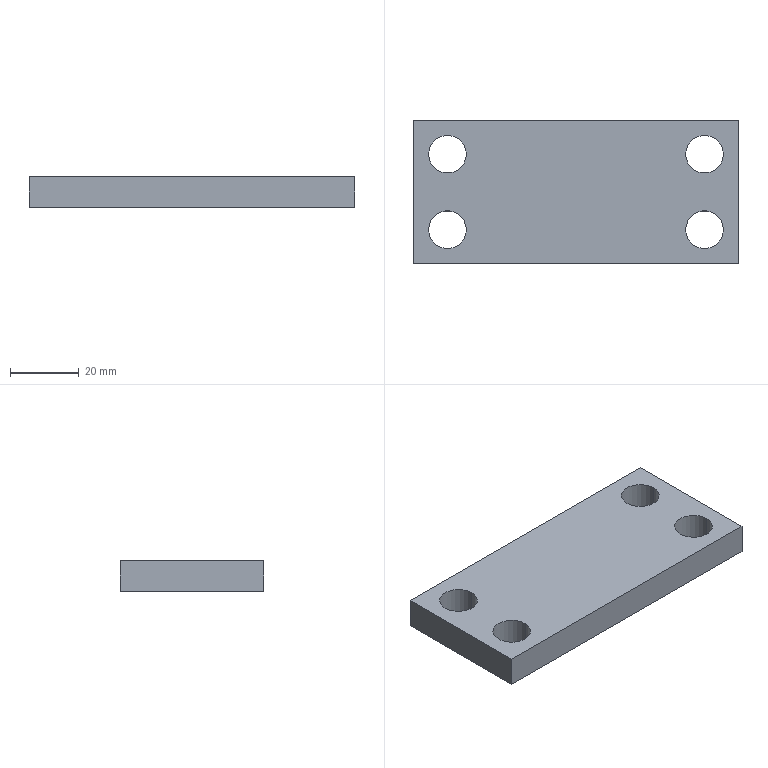Part | STEP file | 0244_203_Spacer | 1 solid | 14 faces | box 95 x 42 x 9 mm | volume 32489 mm3 | cylinder 8 | plane 6 | commonest cylinder face diameters 11 x8
STEP:
#1=CARTESIAN_POINT('',(0.,0.,0.));
#2=DIRECTION('',(0.,0.,1.));
#3=DIRECTION('',(1.,0.,0.));
#4=AXIS2_PLACEMENT_3D('',#1,#2,#3);
#5=CARTESIAN_POINT('',(43.,32.,0.));
#6=VERTEX_POINT('',#5);
#7=CARTESIAN_POINT('',(43.,32.,9.));
#8=VERTEX_POINT('',#7);
#9=CARTESIAN_POINT('',(43.,32.,9.));
#10=DIRECTION('',(0.,0.,1.));
#11=VECTOR('',#10,1.);
#12=LINE('',#9,#11);
#13=CARTESIAN_POINT('',(37.5,32.,9.));
#14=DIRECTION('',(0.,0.,1.));
#15=DIRECTION('',(1.,0.,0.));
#16=AXIS2_PLACEMENT_3D('',#13,#14,#15);
#17=CYLINDRICAL_SURFACE('',#16,5.5);
#18=CARTESIAN_POINT('',(6.283,0.));
#19=DIRECTION('',(0.,1.));
#20=VECTOR('',#19,1.);
#21=LINE('',#18,#20);
#22=(GEOMETRIC_REPRESENTATION_CONTEXT(2)PARAMETRIC_REPRESENTATION_CONTEXT()REPRESENTATION_CONTEXT('',''));
#23=DEFINITIONAL_REPRESENTATION('',(#21),#22);
#24=PCURVE('',#17,#23);
#25=CARTESIAN_POINT('',(37.5,32.,9.));
#26=DIRECTION('',(0.,0.,1.));
#27=DIRECTION('',(1.,0.,0.));
#28=AXIS2_PLACEMENT_3D('',#25,#26,#27);
#29=CYLINDRICAL_SURFACE('',#28,5.5);
#30=CARTESIAN_POINT('',(0.,0.));
#31=DIRECTION('',(0.,1.));
#32=VECTOR('',#31,1.);
#33=LINE('',#30,#32);
#34=(GEOMETRIC_REPRESENTATION_CONTEXT(2)PARAMETRIC_REPRESENTATION_CONTEXT()REPRESENTATION_CONTEXT('',''));
#35=DEFINITIONAL_REPRESENTATION('',(#33),#34);
#36=PCURVE('',#29,#35);
#37=SURFACE_CURVE('',#12,(#24,#36),.PCURVE_S1.);
#38=EDGE_CURVE('',#6,#8,#37,.T.);
#39=ORIENTED_EDGE('',*,*,#38,.T.);
#40=CARTESIAN_POINT('',(32.,32.,9.));
#41=VERTEX_POINT('',#40);
#42=CARTESIAN_POINT('',(37.5,32.,9.));
#43=DIRECTION('',(0.,0.,1.));
#44=DIRECTION('',(1.,0.,0.));
#45=AXIS2_PLACEMENT_3D('',#42,#43,#44);
#46=CIRCLE('',#45,5.5);
#47=CARTESIAN_POINT('',(0.,0.));
#48=DIRECTION('',(1.,0.));
#49=VECTOR('',#48,1.);
#50=LINE('',#47,#49);
#51=(GEOMETRIC_REPRESENTATION_CONTEXT(2)PARAMETRIC_REPRESENTATION_CONTEXT()REPRESENTATION_CONTEXT('',''));
#52=DEFINITIONAL_REPRESENTATION('',(#50),#51);
#53=PCURVE('',#17,#52);
#54=CARTESIAN_POINT('',(-47.5,42.,9.));
#55=DIRECTION('',(0.,0.,-1.));
#56=DIRECTION('',(-1.,0.,0.));
#57=AXIS2_PLACEMENT_3D('',#54,#55,#56);
#58=PLANE('',#57);
#59=CARTESIAN_POINT('',(-90.5,-10.));
#60=CARTESIAN_POINT('',(-90.5,-0.4737));
#61=CARTESIAN_POINT('',(-82.25,-5.237));
#62=CARTESIAN_POINT('',(-74.,-10.));
#63=CARTESIAN_POINT('',(-82.25,-14.763));
#64=CARTESIAN_POINT('',(-90.5,-19.526));
#65=CARTESIAN_POINT('',(-90.5,-10.));
#66=(BOUNDED_CURVE()B_SPLINE_CURVE(2,(#59,#60,#61,#62,#63,#64,#65),.UNSPECIFIED.,.T.,.F.)B_SPLINE_CURVE_WITH_KNOTS((1,2,2,2,2,1),(-2.094,0.,2.094,4.189,6.283,8.378),.UNSPECIFIED.)CURVE()GEOMETRIC_REPRESENTATION_ITEM()RATIONAL_B_SPLINE_CURVE((1.,0.5,1.,0.5,1.,0.5,1.))REPRESENTATION_ITEM(''));
#67=(GEOMETRIC_REPRESENTATION_CONTEXT(2)PARAMETRIC_REPRESENTATION_CONTEXT()REPRESENTATION_CONTEXT('',''));
#68=DEFINITIONAL_REPRESENTATION('',(#66),#67);
#69=PCURVE('',#58,#68);
#70=SURFACE_CURVE('',#46,(#53,#69),.PCURVE_S1.);
#71=EDGE_CURVE('',#41,#8,#70,.T.);
#72=ORIENTED_EDGE('',*,*,#71,.F.);
#73=CARTESIAN_POINT('',(32.,32.,0.));
#74=VERTEX_POINT('',#73);
#75=CARTESIAN_POINT('',(32.,32.,9.));
#76=DIRECTION('',(0.,0.,1.));
#77=VECTOR('',#76,1.);
#78=LINE('',#75,#77);
#79=CARTESIAN_POINT('',(3.142,0.));
#80=DIRECTION('',(0.,1.));
#81=VECTOR('',#80,1.);
#82=LINE('',#79,#81);
#83=(GEOMETRIC_REPRESENTATION_CONTEXT(2)PARAMETRIC_REPRESENTATION_CONTEXT()REPRESENTATION_CONTEXT('',''));
#84=DEFINITIONAL_REPRESENTATION('',(#82),#83);
#85=PCURVE('',#17,#84);
#86=CARTESIAN_POINT('',(3.142,0.));
#87=DIRECTION('',(0.,1.));
#88=VECTOR('',#87,1.);
#89=LINE('',#86,#88);
#90=(GEOMETRIC_REPRESENTATION_CONTEXT(2)PARAMETRIC_REPRESENTATION_CONTEXT()REPRESENTATION_CONTEXT('',''));
#91=DEFINITIONAL_REPRESENTATION('',(#89),#90);
#92=PCURVE('',#29,#91);
#93=SURFACE_CURVE('',#78,(#85,#92),.PCURVE_S1.);
#94=EDGE_CURVE('',#74,#41,#93,.T.);
#95=ORIENTED_EDGE('',*,*,#94,.F.);
#96=CARTESIAN_POINT('',(37.5,32.,0.));
#97=DIRECTION('',(0.,0.,1.));
#98=DIRECTION('',(1.,0.,0.));
#99=AXIS2_PLACEMENT_3D('',#96,#97,#98);
#100=CIRCLE('',#99,5.5);
#101=CARTESIAN_POINT('',(0.,-9.));
#102=DIRECTION('',(1.,0.));
#103=VECTOR('',#102,1.);
#104=LINE('',#101,#103);
#105=(GEOMETRIC_REPRESENTATION_CONTEXT(2)PARAMETRIC_REPRESENTATION_CONTEXT()REPRESENTATION_CONTEXT('',''));
#106=DEFINITIONAL_REPRESENTATION('',(#104),#105);
#107=PCURVE('',#17,#106);
#108=CARTESIAN_POINT('',(-47.5,42.,0.));
#109=DIRECTION('',(0.,0.,-1.));
#110=DIRECTION('',(-1.,0.,0.));
#111=AXIS2_PLACEMENT_3D('',#108,#109,#110);
#112=PLANE('',#111);
#113=CARTESIAN_POINT('',(-90.5,-10.));
#114=CARTESIAN_POINT('',(-90.5,-0.4737));
#115=CARTESIAN_POINT('',(-82.25,-5.237));
#116=CARTESIAN_POINT('',(-74.,-10.));
#117=CARTESIAN_POINT('',(-82.25,-14.763));
#118=CARTESIAN_POINT('',(-90.5,-19.526));
#119=CARTESIAN_POINT('',(-90.5,-10.));
#120=(BOUNDED_CURVE()B_SPLINE_CURVE(2,(#113,#114,#115,#116,#117,#118,#119),.UNSPECIFIED.,.T.,.F.)B_SPLINE_CURVE_WITH_KNOTS((1,2,2,2,2,1),(-2.094,0.,2.094,4.189,6.283,8.378),.UNSPECIFIED.)CURVE()GEOMETRIC_REPRESENTATION_ITEM()RATIONAL_B_SPLINE_CURVE((1.,0.5,1.,0.5,1.,0.5,1.))REPRESENTATION_ITEM(''));
#121=(GEOMETRIC_REPRESENTATION_CONTEXT(2)PARAMETRIC_REPRESENTATION_CONTEXT()REPRESENTATION_CONTEXT('',''));
#122=DEFINITIONAL_REPRESENTATION('',(#120),#121);
#123=PCURVE('',#112,#122);
#124=SURFACE_CURVE('',#100,(#107,#123),.PCURVE_S1.);
#125=EDGE_CURVE('',#74,#6,#124,.T.);
#126=ORIENTED_EDGE('',*,*,#125,.T.);
#127=EDGE_LOOP('',(#39,#72,#95,#126));
#128=FACE_BOUND('',#127,.F.);
#129=ADVANCED_FACE('',(#128),#17,.F.);
#130=CARTESIAN_POINT('',(-32.,32.,0.));
#131=VERTEX_POINT('',#130);
#132=CARTESIAN_POINT('',(-32.,32.,9.));
#133=VERTEX_POINT('',#132);
#134=CARTESIAN_POINT('',(-32.,32.,9.));
#135=DIRECTION('',(0.,0.,1.));
#136=VECTOR('',#135,1.);
#137=LINE('',#134,#136);
#138=CARTESIAN_POINT('',(-37.5,32.,9.));
#139=DIRECTION('',(0.,0.,1.));
#140=DIRECTION('',(1.,0.,0.));
#141=AXIS2_PLACEMENT_3D('',#138,#139,#140);
#142=CYLINDRICAL_SURFACE('',#141,5.5);
#143=CARTESIAN_POINT('',(6.283,0.));
#144=DIRECTION('',(0.,1.));
#145=VECTOR('',#144,1.);
#146=LINE('',#143,#145);
#147=(GEOMETRIC_REPRESENTATION_CONTEXT(2)PARAMETRIC_REPRESENTATION_CONTEXT()REPRESENTATION_CONTEXT('',''));
#148=DEFINITIONAL_REPRESENTATION('',(#146),#147);
#149=PCURVE('',#142,#148);
#150=CARTESIAN_POINT('',(-37.5,32.,9.));
#151=DIRECTION('',(0.,0.,1.));
#152=DIRECTION('',(1.,0.,0.));
#153=AXIS2_PLACEMENT_3D('',#150,#151,#152);
#154=CYLINDRICAL_SURFACE('',#153,5.5);
#155=CARTESIAN_POINT('',(0.,0.));
#156=DIRECTION('',(0.,1.));
#157=VECTOR('',#156,1.);
#158=LINE('',#155,#157);
#159=(GEOMETRIC_REPRESENTATION_CONTEXT(2)PARAMETRIC_REPRESENTATION_CONTEXT()REPRESENTATION_CONTEXT('',''));
#160=DEFINITIONAL_REPRESENTATION('',(#158),#159);
#161=PCURVE('',#154,#160);
#162=SURFACE_CURVE('',#137,(#149,#161),.PCURVE_S1.);
#163=EDGE_CURVE('',#131,#133,#162,.T.);
#164=ORIENTED_EDGE('',*,*,#163,.T.);
#165=CARTESIAN_POINT('',(-43.,32.,9.));
#166=VERTEX_POINT('',#165);
#167=CARTESIAN_POINT('',(-37.5,32.,9.));
#168=DIRECTION('',(0.,0.,1.));
#169=DIRECTION('',(1.,0.,0.));
#170=AXIS2_PLACEMENT_3D('',#167,#168,#169);
#171=CIRCLE('',#170,5.5);
#172=CARTESIAN_POINT('',(0.,0.));
#173=DIRECTION('',(1.,0.));
#174=VECTOR('',#173,1.);
#175=LINE('',#172,#174);
#176=(GEOMETRIC_REPRESENTATION_CONTEXT(2)PARAMETRIC_REPRESENTATION_CONTEXT()REPRESENTATION_CONTEXT('',''));
#177=DEFINITIONAL_REPRESENTATION('',(#175),#176);
#178=PCURVE('',#142,#177);
#179=CARTESIAN_POINT('',(-15.5,-10.));
#180=CARTESIAN_POINT('',(-15.5,-0.4737));
#181=CARTESIAN_POINT('',(-7.25,-5.237));
#182=CARTESIAN_POINT('',(1.,-10.));
#183=CARTESIAN_POINT('',(-7.25,-14.763));
#184=CARTESIAN_POINT('',(-15.5,-19.526));
#185=CARTESIAN_POINT('',(-15.5,-10.));
#186=(BOUNDED_CURVE()B_SPLINE_CURVE(2,(#179,#180,#181,#182,#183,#184,#185),.UNSPECIFIED.,.T.,.F.)B_SPLINE_CURVE_WITH_KNOTS((1,2,2,2,2,1),(-2.094,0.,2.094,4.189,6.283,8.378),.UNSPECIFIED.)CURVE()GEOMETRIC_REPRESENTATION_ITEM()RATIONAL_B_SPLINE_CURVE((1.,0.5,1.,0.5,1.,0.5,1.))REPRESENTATION_ITEM(''));
#187=(GEOMETRIC_REPRESENTATION_CONTEXT(2)PARAMETRIC_REPRESENTATION_CONTEXT()REPRESENTATION_CONTEXT('',''));
#188=DEFINITIONAL_REPRESENTATION('',(#186),#187);
#189=PCURVE('',#58,#188);
#190=SURFACE_CURVE('',#171,(#178,#189),.PCURVE_S1.);
#191=EDGE_CURVE('',#166,#133,#190,.T.);
#192=ORIENTED_EDGE('',*,*,#191,.F.);
#193=CARTESIAN_POINT('',(-43.,32.,0.));
#194=VERTEX_POINT('',#193);
#195=CARTESIAN_POINT('',(-43.,32.,9.));
#196=DIRECTION('',(0.,0.,1.));
#197=VECTOR('',#196,1.);
#198=LINE('',#195,#197);
#199=CARTESIAN_POINT('',(3.142,0.));
#200=DIRECTION('',(0.,1.));
#201=VECTOR('',#200,1.);
#202=LINE('',#199,#201);
#203=(GEOMETRIC_REPRESENTATION_CONTEXT(2)PARAMETRIC_REPRESENTATION_CONTEXT()REPRESENTATION_CONTEXT('',''));
#204=DEFINITIONAL_REPRESENTATION('',(#202),#203);
#205=PCURVE('',#142,#204);
#206=CARTESIAN_POINT('',(3.142,0.));
#207=DIRECTION('',(0.,1.));
#208=VECTOR('',#207,1.);
#209=LINE('',#206,#208);
#210=(GEOMETRIC_REPRESENTATION_CONTEXT(2)PARAMETRIC_REPRESENTATION_CONTEXT()REPRESENTATION_CONTEXT('',''));
#211=DEFINITIONAL_REPRESENTATION('',(#209),#210);
#212=PCURVE('',#154,#211);
#213=SURFACE_CURVE('',#198,(#205,#212),.PCURVE_S1.);
#214=EDGE_CURVE('',#194,#166,#213,.T.);
#215=ORIENTED_EDGE('',*,*,#214,.F.);
#216=CARTESIAN_POINT('',(-37.5,32.,0.));
#217=DIRECTION('',(0.,0.,1.));
#218=DIRECTION('',(1.,0.,0.));
#219=AXIS2_PLACEMENT_3D('',#216,#217,#218);
#220=CIRCLE('',#219,5.5);
#221=CARTESIAN_POINT('',(0.,-9.));
#222=DIRECTION('',(1.,0.));
#223=VECTOR('',#222,1.);
#224=LINE('',#221,#223);
#225=(GEOMETRIC_REPRESENTATION_CONTEXT(2)PARAMETRIC_REPRESENTATION_CONTEXT()REPRESENTATION_CONTEXT('',''));
#226=DEFINITIONAL_REPRESENTATION('',(#224),#225);
#227=PCURVE('',#142,#226);
#228=CARTESIAN_POINT('',(-15.5,-10.));
#229=CARTESIAN_POINT('',(-15.5,-0.4737));
#230=CARTESIAN_POINT('',(-7.25,-5.237));
#231=CARTESIAN_POINT('',(1.,-10.));
#232=CARTESIAN_POINT('',(-7.25,-14.763));
#233=CARTESIAN_POINT('',(-15.5,-19.526));
#234=CARTESIAN_POINT('',(-15.5,-10.));
#235=(BOUNDED_CURVE()B_SPLINE_CURVE(2,(#228,#229,#230,#231,#232,#233,#234),.UNSPECIFIED.,.T.,.F.)B_SPLINE_CURVE_WITH_KNOTS((1,2,2,2,2,1),(-2.094,0.,2.094,4.189,6.283,8.378),.UNSPECIFIED.)CURVE()GEOMETRIC_REPRESENTATION_ITEM()RATIONAL_B_SPLINE_CURVE((1.,0.5,1.,0.5,1.,0.5,1.))REPRESENTATION_ITEM(''));
#236=(GEOMETRIC_REPRESENTATION_CONTEXT(2)PARAMETRIC_REPRESENTATION_CONTEXT()REPRESENTATION_CONTEXT('',''));
#237=DEFINITIONAL_REPRESENTATION('',(#235),#236);
#238=PCURVE('',#112,#237);
#239=SURFACE_CURVE('',#220,(#227,#238),.PCURVE_S1.);
#240=EDGE_CURVE('',#194,#131,#239,.T.);
#241=ORIENTED_EDGE('',*,*,#240,.T.);
#242=EDGE_LOOP('',(#164,#192,#215,#241));
#243=FACE_BOUND('',#242,.F.);
#244=ADVANCED_FACE('',(#243),#142,.F.);
#245=CARTESIAN_POINT('',(43.,10.,0.));
#246=VERTEX_POINT('',#245);
#247=CARTESIAN_POINT('',(43.,10.,9.));
#248=VERTEX_POINT('',#247);
#249=CARTESIAN_POINT('',(43.,10.,9.));
#250=DIRECTION('',(0.,0.,1.));
#251=VECTOR('',#250,1.);
#252=LINE('',#249,#251);
#253=CARTESIAN_POINT('',(37.5,10.,9.));
#254=DIRECTION('',(0.,0.,1.));
#255=DIRECTION('',(1.,0.,0.));
#256=AXIS2_PLACEMENT_3D('',#253,#254,#255);
#257=CYLINDRICAL_SURFACE('',#256,5.5);
#258=CARTESIAN_POINT('',(6.283,0.));
#259=DIRECTION('',(0.,1.));
#260=VECTOR('',#259,1.);
#261=LINE('',#258,#260);
#262=(GEOMETRIC_REPRESENTATION_CONTEXT(2)PARAMETRIC_REPRESENTATION_CONTEXT()REPRESENTATION_CONTEXT('',''));
#263=DEFINITIONAL_REPRESENTATION('',(#261),#262);
#264=PCURVE('',#257,#263);
#265=CARTESIAN_POINT('',(37.5,10.,9.));
#266=DIRECTION('',(0.,0.,1.));
#267=DIRECTION('',(1.,0.,0.));
#268=AXIS2_PLACEMENT_3D('',#265,#266,#267);
#269=CYLINDRICAL_SURFACE('',#268,5.5);
#270=CARTESIAN_POINT('',(0.,0.));
#271=DIRECTION('',(0.,1.));
#272=VECTOR('',#271,1.);
#273=LINE('',#270,#272);
#274=(GEOMETRIC_REPRESENTATION_CONTEXT(2)PARAMETRIC_REPRESENTATION_CONTEXT()REPRESENTATION_CONTEXT('',''));
#275=DEFINITIONAL_REPRESENTATION('',(#273),#274);
#276=PCURVE('',#269,#275);
#277=SURFACE_CURVE('',#252,(#264,#276),.PCURVE_S1.);
#278=EDGE_CURVE('',#246,#248,#277,.T.);
#279=ORIENTED_EDGE('',*,*,#278,.T.);
#280=CARTESIAN_POINT('',(32.,10.,9.));
#281=VERTEX_POINT('',#280);
#282=CARTESIAN_POINT('',(37.5,10.,9.));
#283=DIRECTION('',(0.,0.,1.));
#284=DIRECTION('',(1.,0.,0.));
#285=AXIS2_PLACEMENT_3D('',#282,#283,#284);
#286=CIRCLE('',#285,5.5);
#287=CARTESIAN_POINT('',(0.,0.));
#288=DIRECTION('',(1.,0.));
#289=VECTOR('',#288,1.);
#290=LINE('',#287,#289);
#291=(GEOMETRIC_REPRESENTATION_CONTEXT(2)PARAMETRIC_REPRESENTATION_CONTEXT()REPRESENTATION_CONTEXT('',''));
#292=DEFINITIONAL_REPRESENTATION('',(#290),#291);
#293=PCURVE('',#257,#292);
#294=CARTESIAN_POINT('',(-90.5,-32.));
#295=CARTESIAN_POINT('',(-90.5,-22.474));
#296=CARTESIAN_POINT('',(-82.25,-27.237));
#297=CARTESIAN_POINT('',(-74.,-32.));
#298=CARTESIAN_POINT('',(-82.25,-36.763));
#299=CARTESIAN_POINT('',(-90.5,-41.526));
#300=CARTESIAN_POINT('',(-90.5,-32.));
#301=(BOUNDED_CURVE()B_SPLINE_CURVE(2,(#294,#295,#296,#297,#298,#299,#300),.UNSPECIFIED.,.T.,.F.)B_SPLINE_CURVE_WITH_KNOTS((1,2,2,2,2,1),(-2.094,0.,2.094,4.189,6.283,8.378),.UNSPECIFIED.)CURVE()GEOMETRIC_REPRESENTATION_ITEM()RATIONAL_B_SPLINE_CURVE((1.,0.5,1.,0.5,1.,0.5,1.))REPRESENTATION_ITEM(''));
#302=(GEOMETRIC_REPRESENTATION_CONTEXT(2)PARAMETRIC_REPRESENTATION_CONTEXT()REPRESENTATION_CONTEXT('',''));
#303=DEFINITIONAL_REPRESENTATION('',(#301),#302);
#304=PCURVE('',#58,#303);
#305=SURFACE_CURVE('',#286,(#293,#304),.PCURVE_S1.);
#306=EDGE_CURVE('',#281,#248,#305,.T.);
#307=ORIENTED_EDGE('',*,*,#306,.F.);
#308=CARTESIAN_POINT('',(32.,10.,0.));
#309=VERTEX_POINT('',#308);
#310=CARTESIAN_POINT('',(32.,10.,9.));
#311=DIRECTION('',(0.,0.,1.));
#312=VECTOR('',#311,1.);
#313=LINE('',#310,#312);
#314=CARTESIAN_POINT('',(3.142,0.));
#315=DIRECTION('',(0.,1.));
#316=VECTOR('',#315,1.);
#317=LINE('',#314,#316);
#318=(GEOMETRIC_REPRESENTATION_CONTEXT(2)PARAMETRIC_REPRESENTATION_CONTEXT()REPRESENTATION_CONTEXT('',''));
#319=DEFINITIONAL_REPRESENTATION('',(#317),#318);
#320=PCURVE('',#257,#319);
#321=CARTESIAN_POINT('',(3.142,0.));
#322=DIRECTION('',(0.,1.));
#323=VECTOR('',#322,1.);
#324=LINE('',#321,#323);
#325=(GEOMETRIC_REPRESENTATION_CONTEXT(2)PARAMETRIC_REPRESENTATION_CONTEXT()REPRESENTATION_CONTEXT('',''));
#326=DEFINITIONAL_REPRESENTATION('',(#324),#325);
#327=PCURVE('',#269,#326);
#328=SURFACE_CURVE('',#313,(#320,#327),.PCURVE_S1.);
#329=EDGE_CURVE('',#309,#281,#328,.T.);
#330=ORIENTED_EDGE('',*,*,#329,.F.);
#331=CARTESIAN_POINT('',(37.5,10.,0.));
#332=DIRECTION('',(0.,0.,1.));
#333=DIRECTION('',(1.,0.,0.));
#334=AXIS2_PLACEMENT_3D('',#331,#332,#333);
#335=CIRCLE('',#334,5.5);
#336=CARTESIAN_POINT('',(0.,-9.));
#337=DIRECTION('',(1.,0.));
#338=VECTOR('',#337,1.);
#339=LINE('',#336,#338);
#340=(GEOMETRIC_REPRESENTATION_CONTEXT(2)PARAMETRIC_REPRESENTATION_CONTEXT()REPRESENTATION_CONTEXT('',''));
#341=DEFINITIONAL_REPRESENTATION('',(#339),#340);
#342=PCURVE('',#257,#341);
#343=CARTESIAN_POINT('',(-90.5,-32.));
#344=CARTESIAN_POINT('',(-90.5,-22.474));
#345=CARTESIAN_POINT('',(-82.25,-27.237));
#346=CARTESIAN_POINT('',(-74.,-32.));
#347=CARTESIAN_POINT('',(-82.25,-36.763));
#348=CARTESIAN_POINT('',(-90.5,-41.526));
#349=CARTESIAN_POINT('',(-90.5,-32.));
#350=(BOUNDED_CURVE()B_SPLINE_CURVE(2,(#343,#344,#345,#346,#347,#348,#349),.UNSPECIFIED.,.T.,.F.)B_SPLINE_CURVE_WITH_KNOTS((1,2,2,2,2,1),(-2.094,0.,2.094,4.189,6.283,8.378),.UNSPECIFIED.)CURVE()GEOMETRIC_REPRESENTATION_ITEM()RATIONAL_B_SPLINE_CURVE((1.,0.5,1.,0.5,1.,0.5,1.))REPRESENTATION_ITEM(''));
#351=(GEOMETRIC_REPRESENTATION_CONTEXT(2)PARAMETRIC_REPRESENTATION_CONTEXT()REPRESENTATION_CONTEXT('',''));
#352=DEFINITIONAL_REPRESENTATION('',(#350),#351);
#353=PCURVE('',#112,#352);
#354=SURFACE_CURVE('',#335,(#342,#353),.PCURVE_S1.);
#355=EDGE_CURVE('',#309,#246,#354,.T.);
#356=ORIENTED_EDGE('',*,*,#355,.T.);
#357=EDGE_LOOP('',(#279,#307,#330,#356));
#358=FACE_BOUND('',#357,.F.);
#359=ADVANCED_FACE('',(#358),#257,.F.);
#360=CARTESIAN_POINT('',(-32.,10.,0.));
#361=VERTEX_POINT('',#360);
#362=CARTESIAN_POINT('',(-32.,10.,9.));
#363=VERTEX_POINT('',#362);
#364=CARTESIAN_POINT('',(-32.,10.,9.));
#365=DIRECTION('',(0.,0.,1.));
#366=VECTOR('',#365,1.);
#367=LINE('',#364,#366);
#368=CARTESIAN_POINT('',(-37.5,10.,9.));
#369=DIRECTION('',(0.,0.,1.));
#370=DIRECTION('',(1.,0.,0.));
#371=AXIS2_PLACEMENT_3D('',#368,#369,#370);
#372=CYLINDRICAL_SURFACE('',#371,5.5);
#373=CARTESIAN_POINT('',(6.283,0.));
#374=DIRECTION('',(0.,1.));
#375=VECTOR('',#374,1.);
#376=LINE('',#373,#375);
#377=(GEOMETRIC_REPRESENTATION_CONTEXT(2)PARAMETRIC_REPRESENTATION_CONTEXT()REPRESENTATION_CONTEXT('',''));
#378=DEFINITIONAL_REPRESENTATION('',(#376),#377);
#379=PCURVE('',#372,#378);
#380=CARTESIAN_POINT('',(-37.5,10.,9.));
#381=DIRECTION('',(0.,0.,1.));
#382=DIRECTION('',(1.,0.,0.));
#383=AXIS2_PLACEMENT_3D('',#380,#381,#382);
#384=CYLINDRICAL_SURFACE('',#383,5.5);
#385=CARTESIAN_POINT('',(0.,0.));
#386=DIRECTION('',(0.,1.));
#387=VECTOR('',#386,1.);
#388=LINE('',#385,#387);
#389=(GEOMETRIC_REPRESENTATION_CONTEXT(2)PARAMETRIC_REPRESENTATION_CONTEXT()REPRESENTATION_CONTEXT('',''));
#390=DEFINITIONAL_REPRESENTATION('',(#388),#389);
#391=PCURVE('',#384,#390);
#392=SURFACE_CURVE('',#367,(#379,#391),.PCURVE_S1.);
#393=EDGE_CURVE('',#361,#363,#392,.T.);
#394=ORIENTED_EDGE('',*,*,#393,.T.);
#395=CARTESIAN_POINT('',(-43.,10.,9.));
#396=VERTEX_POINT('',#395);
#397=CARTESIAN_POINT('',(-37.5,10.,9.));
#398=DIRECTION('',(0.,0.,1.));
#399=DIRECTION('',(1.,0.,0.));
#400=AXIS2_PLACEMENT_3D('',#397,#398,#399);
#401=CIRCLE('',#400,5.5);
#402=CARTESIAN_POINT('',(0.,0.));
#403=DIRECTION('',(1.,0.));
#404=VECTOR('',#403,1.);
#405=LINE('',#402,#404);
#406=(GEOMETRIC_REPRESENTATION_CONTEXT(2)PARAMETRIC_REPRESENTATION_CONTEXT()REPRESENTATION_CONTEXT('',''));
#407=DEFINITIONAL_REPRESENTATION('',(#405),#406);
#408=PCURVE('',#372,#407);
#409=CARTESIAN_POINT('',(-15.5,-32.));
#410=CARTESIAN_POINT('',(-15.5,-22.474));
#411=CARTESIAN_POINT('',(-7.25,-27.237));
#412=CARTESIAN_POINT('',(1.,-32.));
#413=CARTESIAN_POINT('',(-7.25,-36.763));
#414=CARTESIAN_POINT('',(-15.5,-41.526));
#415=CARTESIAN_POINT('',(-15.5,-32.));
#416=(BOUNDED_CURVE()B_SPLINE_CURVE(2,(#409,#410,#411,#412,#413,#414,#415),.UNSPECIFIED.,.T.,.F.)B_SPLINE_CURVE_WITH_KNOTS((1,2,2,2,2,1),(-2.094,0.,2.094,4.189,6.283,8.378),.UNSPECIFIED.)CURVE()GEOMETRIC_REPRESENTATION_ITEM()RATIONAL_B_SPLINE_CURVE((1.,0.5,1.,0.5,1.,0.5,1.))REPRESENTATION_ITEM(''));
#417=(GEOMETRIC_REPRESENTATION_CONTEXT(2)PARAMETRIC_REPRESENTATION_CONTEXT()REPRESENTATION_CONTEXT('',''));
#418=DEFINITIONAL_REPRESENTATION('',(#416),#417);
#419=PCURVE('',#58,#418);
#420=SURFACE_CURVE('',#401,(#408,#419),.PCURVE_S1.);
#421=EDGE_CURVE('',#396,#363,#420,.T.);
#422=ORIENTED_EDGE('',*,*,#421,.F.);
#423=CARTESIAN_POINT('',(-43.,10.,0.));
#424=VERTEX_POINT('',#423);
#425=CARTESIAN_POINT('',(-43.,10.,9.));
#426=DIRECTION('',(0.,0.,1.));
#427=VECTOR('',#426,1.);
#428=LINE('',#425,#427);
#429=CARTESIAN_POINT('',(3.142,0.));
#430=DIRECTION('',(0.,1.));
#431=VECTOR('',#430,1.);
#432=LINE('',#429,#431);
#433=(GEOMETRIC_REPRESENTATION_CONTEXT(2)PARAMETRIC_REPRESENTATION_CONTEXT()REPRESENTATION_CONTEXT('',''));
#434=DEFINITIONAL_REPRESENTATION('',(#432),#433);
#435=PCURVE('',#372,#434);
#436=CARTESIAN_POINT('',(3.142,0.));
#437=DIRECTION('',(0.,1.));
#438=VECTOR('',#437,1.);
#439=LINE('',#436,#438);
#440=(GEOMETRIC_REPRESENTATION_CONTEXT(2)PARAMETRIC_REPRESENTATION_CONTEXT()REPRESENTATION_CONTEXT('',''));
#441=DEFINITIONAL_REPRESENTATION('',(#439),#440);
#442=PCURVE('',#384,#441);
#443=SURFACE_CURVE('',#428,(#435,#442),.PCURVE_S1.);
#444=EDGE_CURVE('',#424,#396,#443,.T.);
#445=ORIENTED_EDGE('',*,*,#444,.F.);
#446=CARTESIAN_POINT('',(-37.5,10.,0.));
#447=DIRECTION('',(0.,0.,1.));
#448=DIRECTION('',(1.,0.,0.));
#449=AXIS2_PLACEMENT_3D('',#446,#447,#448);
#450=CIRCLE('',#449,5.5);
#451=CARTESIAN_POINT('',(0.,-9.));
#452=DIRECTION('',(1.,0.));
#453=VECTOR('',#452,1.);
#454=LINE('',#451,#453);
#455=(GEOMETRIC_REPRESENTATION_CONTEXT(2)PARAMETRIC_REPRESENTATION_CONTEXT()REPRESENTATION_CONTEXT('',''));
#456=DEFINITIONAL_REPRESENTATION('',(#454),#455);
#457=PCURVE('',#372,#456);
#458=CARTESIAN_POINT('',(-15.5,-32.));
#459=CARTESIAN_POINT('',(-15.5,-22.474));
#460=CARTESIAN_POINT('',(-7.25,-27.237));
#461=CARTESIAN_POINT('',(1.,-32.));
#462=CARTESIAN_POINT('',(-7.25,-36.763));
#463=CARTESIAN_POINT('',(-15.5,-41.526));
#464=CARTESIAN_POINT('',(-15.5,-32.));
#465=(BOUNDED_CURVE()B_SPLINE_CURVE(2,(#458,#459,#460,#461,#462,#463,#464),.UNSPECIFIED.,.T.,.F.)B_SPLINE_CURVE_WITH_KNOTS((1,2,2,2,2,1),(-2.094,0.,2.094,4.189,6.283,8.378),.UNSPECIFIED.)CURVE()GEOMETRIC_REPRESENTATION_ITEM()RATIONAL_B_SPLINE_CURVE((1.,0.5,1.,0.5,1.,0.5,1.))REPRESENTATION_ITEM(''));
#466=(GEOMETRIC_REPRESENTATION_CONTEXT(2)PARAMETRIC_REPRESENTATION_CONTEXT()REPRESENTATION_CONTEXT('',''));
#467=DEFINITIONAL_REPRESENTATION('',(#465),#466);
#468=PCURVE('',#112,#467);
#469=SURFACE_CURVE('',#450,(#457,#468),.PCURVE_S1.);
#470=EDGE_CURVE('',#424,#361,#469,.T.);
#471=ORIENTED_EDGE('',*,*,#470,.T.);
#472=EDGE_LOOP('',(#394,#422,#445,#471));
#473=FACE_BOUND('',#472,.F.);
#474=ADVANCED_FACE('',(#473),#372,.F.);
#475=CARTESIAN_POINT('',(-47.5,42.,0.));
#476=VERTEX_POINT('',#475);
#477=CARTESIAN_POINT('',(-47.5,0.,0.));
#478=VERTEX_POINT('',#477);
#479=CARTESIAN_POINT('',(-47.5,0.,0.));
#480=DIRECTION('',(0.,-1.,0.));
#481=VECTOR('',#480,1.);
#482=LINE('',#479,#481);
#483=CARTESIAN_POINT('',(-47.5,0.,9.));
#484=DIRECTION('',(1.,0.,0.));
#485=DIRECTION('',(0.,0.,-1.));
#486=AXIS2_PLACEMENT_3D('',#483,#484,#485);
#487=PLANE('',#486);
#488=CARTESIAN_POINT('',(9.,0.));
#489=DIRECTION('',(0.,-1.));
#490=VECTOR('',#489,1.);
#491=LINE('',#488,#490);
#492=(GEOMETRIC_REPRESENTATION_CONTEXT(2)PARAMETRIC_REPRESENTATION_CONTEXT()REPRESENTATION_CONTEXT('',''));
#493=DEFINITIONAL_REPRESENTATION('',(#491),#492);
#494=PCURVE('',#487,#493);
#495=CARTESIAN_POINT('',(0.,-42.));
#496=DIRECTION('',(0.,-1.));
#497=VECTOR('',#496,1.);
#498=LINE('',#495,#497);
#499=(GEOMETRIC_REPRESENTATION_CONTEXT(2)PARAMETRIC_REPRESENTATION_CONTEXT()REPRESENTATION_CONTEXT('',''));
#500=DEFINITIONAL_REPRESENTATION('',(#498),#499);
#501=PCURVE('',#112,#500);
#502=SURFACE_CURVE('',#482,(#494,#501),.PCURVE_S1.);
#503=EDGE_CURVE('',#476,#478,#502,.T.);
#504=ORIENTED_EDGE('',*,*,#503,.T.);
#505=CARTESIAN_POINT('',(-47.5,0.,9.));
#506=VERTEX_POINT('',#505);
#507=CARTESIAN_POINT('',(-47.5,0.,9.));
#508=DIRECTION('',(0.,0.,-1.));
#509=VECTOR('',#508,1.);
#510=LINE('',#507,#509);
#511=CARTESIAN_POINT('',(0.,0.));
#512=DIRECTION('',(1.,0.));
#513=VECTOR('',#512,1.);
#514=LINE('',#511,#513);
#515=(GEOMETRIC_REPRESENTATION_CONTEXT(2)PARAMETRIC_REPRESENTATION_CONTEXT()REPRESENTATION_CONTEXT('',''));
#516=DEFINITIONAL_REPRESENTATION('',(#514),#515);
#517=PCURVE('',#487,#516);
#518=CARTESIAN_POINT('',(-47.5,0.,9.));
#519=DIRECTION('',(0.,1.,0.));
#520=DIRECTION('',(0.,0.,1.));
#521=AXIS2_PLACEMENT_3D('',#518,#519,#520);
#522=PLANE('',#521);
#523=CARTESIAN_POINT('',(0.,0.));
#524=DIRECTION('',(-1.,0.));
#525=VECTOR('',#524,1.);
#526=LINE('',#523,#525);
#527=(GEOMETRIC_REPRESENTATION_CONTEXT(2)PARAMETRIC_REPRESENTATION_CONTEXT()REPRESENTATION_CONTEXT('',''));
#528=DEFINITIONAL_REPRESENTATION('',(#526),#527);
#529=PCURVE('',#522,#528);
#530=SURFACE_CURVE('',#510,(#517,#529),.PCURVE_S1.);
#531=EDGE_CURVE('',#506,#478,#530,.T.);
#532=ORIENTED_EDGE('',*,*,#531,.F.);
#533=CARTESIAN_POINT('',(-47.5,42.,9.));
#534=VERTEX_POINT('',#533);
#535=CARTESIAN_POINT('',(-47.5,0.,9.));
#536=DIRECTION('',(0.,-1.,0.));
#537=VECTOR('',#536,1.);
#538=LINE('',#535,#537);
#539=CARTESIAN_POINT('',(0.,0.));
#540=DIRECTION('',(0.,-1.));
#541=VECTOR('',#540,1.);
#542=LINE('',#539,#541);
#543=(GEOMETRIC_REPRESENTATION_CONTEXT(2)PARAMETRIC_REPRESENTATION_CONTEXT()REPRESENTATION_CONTEXT('',''));
#544=DEFINITIONAL_REPRESENTATION('',(#542),#543);
#545=PCURVE('',#487,#544);
#546=CARTESIAN_POINT('',(0.,-42.));
#547=DIRECTION('',(0.,-1.));
#548=VECTOR('',#547,1.);
#549=LINE('',#546,#548);
#550=(GEOMETRIC_REPRESENTATION_CONTEXT(2)PARAMETRIC_REPRESENTATION_CONTEXT()REPRESENTATION_CONTEXT('',''));
#551=DEFINITIONAL_REPRESENTATION('',(#549),#550);
#552=PCURVE('',#58,#551);
#553=SURFACE_CURVE('',#538,(#545,#552),.PCURVE_S1.);
#554=EDGE_CURVE('',#534,#506,#553,.T.);
#555=ORIENTED_EDGE('',*,*,#554,.F.);
#556=CARTESIAN_POINT('',(-47.5,42.,9.));
#557=DIRECTION('',(0.,0.,-1.));
#558=VECTOR('',#557,1.);
#559=LINE('',#556,#558);
#560=CARTESIAN_POINT('',(0.,42.));
#561=DIRECTION('',(1.,0.));
#562=VECTOR('',#561,1.);
#563=LINE('',#560,#562);
#564=(GEOMETRIC_REPRESENTATION_CONTEXT(2)PARAMETRIC_REPRESENTATION_CONTEXT()REPRESENTATION_CONTEXT('',''));
#565=DEFINITIONAL_REPRESENTATION('',(#563),#564);
#566=PCURVE('',#487,#565);
#567=CARTESIAN_POINT('',(-47.5,42.,9.));
#568=DIRECTION('',(0.,-1.,0.));
#569=DIRECTION('',(0.,0.,-1.));
#570=AXIS2_PLACEMENT_3D('',#567,#568,#569);
#571=PLANE('',#570);
#572=CARTESIAN_POINT('',(0.,0.));
#573=DIRECTION('',(1.,0.));
#574=VECTOR('',#573,1.);
#575=LINE('',#572,#574);
#576=(GEOMETRIC_REPRESENTATION_CONTEXT(2)PARAMETRIC_REPRESENTATION_CONTEXT()REPRESENTATION_CONTEXT('',''));
#577=DEFINITIONAL_REPRESENTATION('',(#575),#576);
#578=PCURVE('',#571,#577);
#579=SURFACE_CURVE('',#559,(#566,#578),.PCURVE_S1.);
#580=EDGE_CURVE('',#534,#476,#579,.T.);
#581=ORIENTED_EDGE('',*,*,#580,.T.);
#582=EDGE_LOOP('',(#504,#532,#555,#581));
#583=FACE_BOUND('',#582,.T.);
#584=ADVANCED_FACE('',(#583),#487,.F.);
#585=CARTESIAN_POINT('',(47.5,0.,0.));
#586=VERTEX_POINT('',#585);
#587=CARTESIAN_POINT('',(-47.5,0.,0.));
#588=DIRECTION('',(1.,0.,0.));
#589=VECTOR('',#588,1.);
#590=LINE('',#587,#589);
#591=CARTESIAN_POINT('',(-9.,0.));
#592=DIRECTION('',(0.,1.));
#593=VECTOR('',#592,1.);
#594=LINE('',#591,#593);
#595=(GEOMETRIC_REPRESENTATION_CONTEXT(2)PARAMETRIC_REPRESENTATION_CONTEXT()REPRESENTATION_CONTEXT('',''));
#596=DEFINITIONAL_REPRESENTATION('',(#594),#595);
#597=PCURVE('',#522,#596);
#598=CARTESIAN_POINT('',(0.,-42.));
#599=DIRECTION('',(-1.,0.));
#600=VECTOR('',#599,1.);
#601=LINE('',#598,#600);
#602=(GEOMETRIC_REPRESENTATION_CONTEXT(2)PARAMETRIC_REPRESENTATION_CONTEXT()REPRESENTATION_CONTEXT('',''));
#603=DEFINITIONAL_REPRESENTATION('',(#601),#602);
#604=PCURVE('',#112,#603);
#605=SURFACE_CURVE('',#590,(#597,#604),.PCURVE_S1.);
#606=EDGE_CURVE('',#478,#586,#605,.T.);
#607=ORIENTED_EDGE('',*,*,#606,.T.);
#608=CARTESIAN_POINT('',(47.5,0.,9.));
#609=VERTEX_POINT('',#608);
#610=CARTESIAN_POINT('',(47.5,0.,9.));
#611=DIRECTION('',(0.,0.,-1.));
#612=VECTOR('',#611,1.);
#613=LINE('',#610,#612);
#614=CARTESIAN_POINT('',(0.,95.));
#615=DIRECTION('',(-1.,0.));
#616=VECTOR('',#615,1.);
#617=LINE('',#614,#616);
#618=(GEOMETRIC_REPRESENTATION_CONTEXT(2)PARAMETRIC_REPRESENTATION_CONTEXT()REPRESENTATION_CONTEXT('',''));
#619=DEFINITIONAL_REPRESENTATION('',(#617),#618);
#620=PCURVE('',#522,#619);
#621=CARTESIAN_POINT('',(47.5,0.,9.));
#622=DIRECTION('',(-1.,0.,0.));
#623=DIRECTION('',(0.,0.,1.));
#624=AXIS2_PLACEMENT_3D('',#621,#622,#623);
#625=PLANE('',#624);
#626=CARTESIAN_POINT('',(0.,0.));
#627=DIRECTION('',(-1.,0.));
#628=VECTOR('',#627,1.);
#629=LINE('',#626,#628);
#630=(GEOMETRIC_REPRESENTATION_CONTEXT(2)PARAMETRIC_REPRESENTATION_CONTEXT()REPRESENTATION_CONTEXT('',''));
#631=DEFINITIONAL_REPRESENTATION('',(#629),#630);
#632=PCURVE('',#625,#631);
#633=SURFACE_CURVE('',#613,(#620,#632),.PCURVE_S1.);
#634=EDGE_CURVE('',#609,#586,#633,.T.);
#635=ORIENTED_EDGE('',*,*,#634,.F.);
#636=CARTESIAN_POINT('',(-47.5,0.,9.));
#637=DIRECTION('',(1.,0.,0.));
#638=VECTOR('',#637,1.);
#639=LINE('',#636,#638);
#640=CARTESIAN_POINT('',(0.,0.));
#641=DIRECTION('',(0.,1.));
#642=VECTOR('',#641,1.);
#643=LINE('',#640,#642);
#644=(GEOMETRIC_REPRESENTATION_CONTEXT(2)PARAMETRIC_REPRESENTATION_CONTEXT()REPRESENTATION_CONTEXT('',''));
#645=DEFINITIONAL_REPRESENTATION('',(#643),#644);
#646=PCURVE('',#522,#645);
#647=CARTESIAN_POINT('',(0.,-42.));
#648=DIRECTION('',(-1.,0.));
#649=VECTOR('',#648,1.);
#650=LINE('',#647,#649);
#651=(GEOMETRIC_REPRESENTATION_CONTEXT(2)PARAMETRIC_REPRESENTATION_CONTEXT()REPRESENTATION_CONTEXT('',''));
#652=DEFINITIONAL_REPRESENTATION('',(#650),#651);
#653=PCURVE('',#58,#652);
#654=SURFACE_CURVE('',#639,(#646,#653),.PCURVE_S1.);
#655=EDGE_CURVE('',#506,#609,#654,.T.);
#656=ORIENTED_EDGE('',*,*,#655,.F.);
#657=ORIENTED_EDGE('',*,*,#531,.T.);
#658=EDGE_LOOP('',(#607,#635,#656,#657));
#659=FACE_BOUND('',#658,.T.);
#660=ADVANCED_FACE('',(#659),#522,.F.);
#661=CARTESIAN_POINT('',(47.5,42.,0.));
#662=VERTEX_POINT('',#661);
#663=CARTESIAN_POINT('',(47.5,0.,0.));
#664=DIRECTION('',(0.,1.,0.));
#665=VECTOR('',#664,1.);
#666=LINE('',#663,#665);
#667=CARTESIAN_POINT('',(-9.,0.));
#668=DIRECTION('',(0.,1.));
#669=VECTOR('',#668,1.);
#670=LINE('',#667,#669);
#671=(GEOMETRIC_REPRESENTATION_CONTEXT(2)PARAMETRIC_REPRESENTATION_CONTEXT()REPRESENTATION_CONTEXT('',''));
#672=DEFINITIONAL_REPRESENTATION('',(#670),#671);
#673=PCURVE('',#625,#672);
#674=CARTESIAN_POINT('',(-95.,-42.));
#675=DIRECTION('',(0.,1.));
#676=VECTOR('',#675,1.);
#677=LINE('',#674,#676);
#678=(GEOMETRIC_REPRESENTATION_CONTEXT(2)PARAMETRIC_REPRESENTATION_CONTEXT()REPRESENTATION_CONTEXT('',''));
#679=DEFINITIONAL_REPRESENTATION('',(#677),#678);
#680=PCURVE('',#112,#679);
#681=SURFACE_CURVE('',#666,(#673,#680),.PCURVE_S1.);
#682=EDGE_CURVE('',#586,#662,#681,.T.);
#683=ORIENTED_EDGE('',*,*,#682,.T.);
#684=CARTESIAN_POINT('',(47.5,42.,9.));
#685=VERTEX_POINT('',#684);
#686=CARTESIAN_POINT('',(47.5,42.,9.));
#687=DIRECTION('',(0.,0.,-1.));
#688=VECTOR('',#687,1.);
#689=LINE('',#686,#688);
#690=CARTESIAN_POINT('',(0.,42.));
#691=DIRECTION('',(-1.,0.));
#692=VECTOR('',#691,1.);
#693=LINE('',#690,#692);
#694=(GEOMETRIC_REPRESENTATION_CONTEXT(2)PARAMETRIC_REPRESENTATION_CONTEXT()REPRESENTATION_CONTEXT('',''));
#695=DEFINITIONAL_REPRESENTATION('',(#693),#694);
#696=PCURVE('',#625,#695);
#697=CARTESIAN_POINT('',(0.,95.));
#698=DIRECTION('',(1.,0.));
#699=VECTOR('',#698,1.);
#700=LINE('',#697,#699);
#701=(GEOMETRIC_REPRESENTATION_CONTEXT(2)PARAMETRIC_REPRESENTATION_CONTEXT()REPRESENTATION_CONTEXT('',''));
#702=DEFINITIONAL_REPRESENTATION('',(#700),#701);
#703=PCURVE('',#571,#702);
#704=SURFACE_CURVE('',#689,(#696,#703),.PCURVE_S1.);
#705=EDGE_CURVE('',#685,#662,#704,.T.);
#706=ORIENTED_EDGE('',*,*,#705,.F.);
#707=CARTESIAN_POINT('',(47.5,0.,9.));
#708=DIRECTION('',(0.,1.,0.));
#709=VECTOR('',#708,1.);
#710=LINE('',#707,#709);
#711=CARTESIAN_POINT('',(0.,0.));
#712=DIRECTION('',(0.,1.));
#713=VECTOR('',#712,1.);
#714=LINE('',#711,#713);
#715=(GEOMETRIC_REPRESENTATION_CONTEXT(2)PARAMETRIC_REPRESENTATION_CONTEXT()REPRESENTATION_CONTEXT('',''));
#716=DEFINITIONAL_REPRESENTATION('',(#714),#715);
#717=PCURVE('',#625,#716);
#718=CARTESIAN_POINT('',(-95.,-42.));
#719=DIRECTION('',(0.,1.));
#720=VECTOR('',#719,1.);
#721=LINE('',#718,#720);
#722=(GEOMETRIC_REPRESENTATION_CONTEXT(2)PARAMETRIC_REPRESENTATION_CONTEXT()REPRESENTATION_CONTEXT('',''));
#723=DEFINITIONAL_REPRESENTATION('',(#721),#722);
#724=PCURVE('',#58,#723);
#725=SURFACE_CURVE('',#710,(#717,#724),.PCURVE_S1.);
#726=EDGE_CURVE('',#609,#685,#725,.T.);
#727=ORIENTED_EDGE('',*,*,#726,.F.);
#728=ORIENTED_EDGE('',*,*,#634,.T.);
#729=EDGE_LOOP('',(#683,#706,#727,#728));
#730=FACE_BOUND('',#729,.T.);
#731=ADVANCED_FACE('',(#730),#625,.F.);
#732=CARTESIAN_POINT('',(-47.5,42.,0.));
#733=DIRECTION('',(-1.,0.,0.));
#734=VECTOR('',#733,1.);
#735=LINE('',#732,#734);
#736=CARTESIAN_POINT('',(9.,0.));
#737=DIRECTION('',(0.,-1.));
#738=VECTOR('',#737,1.);
#739=LINE('',#736,#738);
#740=(GEOMETRIC_REPRESENTATION_CONTEXT(2)PARAMETRIC_REPRESENTATION_CONTEXT()REPRESENTATION_CONTEXT('',''));
#741=DEFINITIONAL_REPRESENTATION('',(#739),#740);
#742=PCURVE('',#571,#741);
#743=CARTESIAN_POINT('',(0.,0.));
#744=DIRECTION('',(1.,0.));
#745=VECTOR('',#744,1.);
#746=LINE('',#743,#745);
#747=(GEOMETRIC_REPRESENTATION_CONTEXT(2)PARAMETRIC_REPRESENTATION_CONTEXT()REPRESENTATION_CONTEXT('',''));
#748=DEFINITIONAL_REPRESENTATION('',(#746),#747);
#749=PCURVE('',#112,#748);
#750=SURFACE_CURVE('',#735,(#742,#749),.PCURVE_S1.);
#751=EDGE_CURVE('',#662,#476,#750,.T.);
#752=ORIENTED_EDGE('',*,*,#751,.T.);
#753=ORIENTED_EDGE('',*,*,#580,.F.);
#754=CARTESIAN_POINT('',(-47.5,42.,9.));
#755=DIRECTION('',(-1.,0.,0.));
#756=VECTOR('',#755,1.);
#757=LINE('',#754,#756);
#758=CARTESIAN_POINT('',(0.,0.));
#759=DIRECTION('',(0.,-1.));
#760=VECTOR('',#759,1.);
#761=LINE('',#758,#760);
#762=(GEOMETRIC_REPRESENTATION_CONTEXT(2)PARAMETRIC_REPRESENTATION_CONTEXT()REPRESENTATION_CONTEXT('',''));
#763=DEFINITIONAL_REPRESENTATION('',(#761),#762);
#764=PCURVE('',#571,#763);
#765=CARTESIAN_POINT('',(0.,0.));
#766=DIRECTION('',(1.,0.));
#767=VECTOR('',#766,1.);
#768=LINE('',#765,#767);
#769=(GEOMETRIC_REPRESENTATION_CONTEXT(2)PARAMETRIC_REPRESENTATION_CONTEXT()REPRESENTATION_CONTEXT('',''));
#770=DEFINITIONAL_REPRESENTATION('',(#768),#769);
#771=PCURVE('',#58,#770);
#772=SURFACE_CURVE('',#757,(#764,#771),.PCURVE_S1.);
#773=EDGE_CURVE('',#685,#534,#772,.T.);
#774=ORIENTED_EDGE('',*,*,#773,.F.);
#775=ORIENTED_EDGE('',*,*,#705,.T.);
#776=EDGE_LOOP('',(#752,#753,#774,#775));
#777=FACE_BOUND('',#776,.T.);
#778=ADVANCED_FACE('',(#777),#571,.F.);
#779=CARTESIAN_POINT('',(37.5,10.,9.));
#780=DIRECTION('',(0.,0.,1.));
#781=DIRECTION('',(1.,0.,0.));
#782=AXIS2_PLACEMENT_3D('',#779,#780,#781);
#783=CIRCLE('',#782,5.5);
#784=CARTESIAN_POINT('',(-90.5,-32.));
#785=CARTESIAN_POINT('',(-90.5,-22.474));
#786=CARTESIAN_POINT('',(-82.25,-27.237));
#787=CARTESIAN_POINT('',(-74.,-32.));
#788=CARTESIAN_POINT('',(-82.25,-36.763));
#789=CARTESIAN_POINT('',(-90.5,-41.526));
#790=CARTESIAN_POINT('',(-90.5,-32.));
#791=(BOUNDED_CURVE()B_SPLINE_CURVE(2,(#784,#785,#786,#787,#788,#789,#790),.UNSPECIFIED.,.T.,.F.)B_SPLINE_CURVE_WITH_KNOTS((1,2,2,2,2,1),(-2.094,0.,2.094,4.189,6.283,8.378),.UNSPECIFIED.)CURVE()GEOMETRIC_REPRESENTATION_ITEM()RATIONAL_B_SPLINE_CURVE((1.,0.5,1.,0.5,1.,0.5,1.))REPRESENTATION_ITEM(''));
#792=(GEOMETRIC_REPRESENTATION_CONTEXT(2)PARAMETRIC_REPRESENTATION_CONTEXT()REPRESENTATION_CONTEXT('',''));
#793=DEFINITIONAL_REPRESENTATION('',(#791),#792);
#794=PCURVE('',#58,#793);
#795=CARTESIAN_POINT('',(0.,0.));
#796=DIRECTION('',(1.,0.));
#797=VECTOR('',#796,1.);
#798=LINE('',#795,#797);
#799=(GEOMETRIC_REPRESENTATION_CONTEXT(2)PARAMETRIC_REPRESENTATION_CONTEXT()REPRESENTATION_CONTEXT('',''));
#800=DEFINITIONAL_REPRESENTATION('',(#798),#799);
#801=PCURVE('',#269,#800);
#802=SURFACE_CURVE('',#783,(#794,#801),.PCURVE_S1.);
#803=EDGE_CURVE('',#248,#281,#802,.T.);
#804=ORIENTED_EDGE('',*,*,#803,.F.);
#805=ORIENTED_EDGE('',*,*,#306,.F.);
#806=EDGE_LOOP('',(#804,#805));
#807=FACE_BOUND('',#806,.T.);
#808=CARTESIAN_POINT('',(-37.5,10.,9.));
#809=DIRECTION('',(0.,0.,1.));
#810=DIRECTION('',(1.,0.,0.));
#811=AXIS2_PLACEMENT_3D('',#808,#809,#810);
#812=CIRCLE('',#811,5.5);
#813=CARTESIAN_POINT('',(-15.5,-32.));
#814=CARTESIAN_POINT('',(-15.5,-22.474));
#815=CARTESIAN_POINT('',(-7.25,-27.237));
#816=CARTESIAN_POINT('',(1.,-32.));
#817=CARTESIAN_POINT('',(-7.25,-36.763));
#818=CARTESIAN_POINT('',(-15.5,-41.526));
#819=CARTESIAN_POINT('',(-15.5,-32.));
#820=(BOUNDED_CURVE()B_SPLINE_CURVE(2,(#813,#814,#815,#816,#817,#818,#819),.UNSPECIFIED.,.T.,.F.)B_SPLINE_CURVE_WITH_KNOTS((1,2,2,2,2,1),(-2.094,0.,2.094,4.189,6.283,8.378),.UNSPECIFIED.)CURVE()GEOMETRIC_REPRESENTATION_ITEM()RATIONAL_B_SPLINE_CURVE((1.,0.5,1.,0.5,1.,0.5,1.))REPRESENTATION_ITEM(''));
#821=(GEOMETRIC_REPRESENTATION_CONTEXT(2)PARAMETRIC_REPRESENTATION_CONTEXT()REPRESENTATION_CONTEXT('',''));
#822=DEFINITIONAL_REPRESENTATION('',(#820),#821);
#823=PCURVE('',#58,#822);
#824=CARTESIAN_POINT('',(0.,0.));
#825=DIRECTION('',(1.,0.));
#826=VECTOR('',#825,1.);
#827=LINE('',#824,#826);
#828=(GEOMETRIC_REPRESENTATION_CONTEXT(2)PARAMETRIC_REPRESENTATION_CONTEXT()REPRESENTATION_CONTEXT('',''));
#829=DEFINITIONAL_REPRESENTATION('',(#827),#828);
#830=PCURVE('',#384,#829);
#831=SURFACE_CURVE('',#812,(#823,#830),.PCURVE_S1.);
#832=EDGE_CURVE('',#363,#396,#831,.T.);
#833=ORIENTED_EDGE('',*,*,#832,.F.);
#834=ORIENTED_EDGE('',*,*,#421,.F.);
#835=EDGE_LOOP('',(#833,#834));
#836=FACE_BOUND('',#835,.T.);
#837=ORIENTED_EDGE('',*,*,#554,.T.);
#838=ORIENTED_EDGE('',*,*,#655,.T.);
#839=ORIENTED_EDGE('',*,*,#726,.T.);
#840=ORIENTED_EDGE('',*,*,#773,.T.);
#841=EDGE_LOOP('',(#837,#838,#839,#840));
#842=FACE_BOUND('',#841,.T.);
#843=CARTESIAN_POINT('',(-37.5,32.,9.));
#844=DIRECTION('',(0.,0.,1.));
#845=DIRECTION('',(1.,0.,0.));
#846=AXIS2_PLACEMENT_3D('',#843,#844,#845);
#847=CIRCLE('',#846,5.5);
#848=CARTESIAN_POINT('',(-15.5,-10.));
#849=CARTESIAN_POINT('',(-15.5,-0.4737));
#850=CARTESIAN_POINT('',(-7.25,-5.237));
#851=CARTESIAN_POINT('',(1.,-10.));
#852=CARTESIAN_POINT('',(-7.25,-14.763));
#853=CARTESIAN_POINT('',(-15.5,-19.526));
#854=CARTESIAN_POINT('',(-15.5,-10.));
#855=(BOUNDED_CURVE()B_SPLINE_CURVE(2,(#848,#849,#850,#851,#852,#853,#854),.UNSPECIFIED.,.T.,.F.)B_SPLINE_CURVE_WITH_KNOTS((1,2,2,2,2,1),(-2.094,0.,2.094,4.189,6.283,8.378),.UNSPECIFIED.)CURVE()GEOMETRIC_REPRESENTATION_ITEM()RATIONAL_B_SPLINE_CURVE((1.,0.5,1.,0.5,1.,0.5,1.))REPRESENTATION_ITEM(''));
#856=(GEOMETRIC_REPRESENTATION_CONTEXT(2)PARAMETRIC_REPRESENTATION_CONTEXT()REPRESENTATION_CONTEXT('',''));
#857=DEFINITIONAL_REPRESENTATION('',(#855),#856);
#858=PCURVE('',#58,#857);
#859=CARTESIAN_POINT('',(0.,0.));
#860=DIRECTION('',(1.,0.));
#861=VECTOR('',#860,1.);
#862=LINE('',#859,#861);
#863=(GEOMETRIC_REPRESENTATION_CONTEXT(2)PARAMETRIC_REPRESENTATION_CONTEXT()REPRESENTATION_CONTEXT('',''));
#864=DEFINITIONAL_REPRESENTATION('',(#862),#863);
#865=PCURVE('',#154,#864);
#866=SURFACE_CURVE('',#847,(#858,#865),.PCURVE_S1.);
#867=EDGE_CURVE('',#133,#166,#866,.T.);
#868=ORIENTED_EDGE('',*,*,#867,.F.);
#869=ORIENTED_EDGE('',*,*,#191,.F.);
#870=EDGE_LOOP('',(#868,#869));
#871=FACE_BOUND('',#870,.T.);
#872=CARTESIAN_POINT('',(37.5,32.,9.));
#873=DIRECTION('',(0.,0.,1.));
#874=DIRECTION('',(1.,0.,0.));
#875=AXIS2_PLACEMENT_3D('',#872,#873,#874);
#876=CIRCLE('',#875,5.5);
#877=CARTESIAN_POINT('',(-90.5,-10.));
#878=CARTESIAN_POINT('',(-90.5,-0.4737));
#879=CARTESIAN_POINT('',(-82.25,-5.237));
#880=CARTESIAN_POINT('',(-74.,-10.));
#881=CARTESIAN_POINT('',(-82.25,-14.763));
#882=CARTESIAN_POINT('',(-90.5,-19.526));
#883=CARTESIAN_POINT('',(-90.5,-10.));
#884=(BOUNDED_CURVE()B_SPLINE_CURVE(2,(#877,#878,#879,#880,#881,#882,#883),.UNSPECIFIED.,.T.,.F.)B_SPLINE_CURVE_WITH_KNOTS((1,2,2,2,2,1),(-2.094,0.,2.094,4.189,6.283,8.378),.UNSPECIFIED.)CURVE()GEOMETRIC_REPRESENTATION_ITEM()RATIONAL_B_SPLINE_CURVE((1.,0.5,1.,0.5,1.,0.5,1.))REPRESENTATION_ITEM(''));
#885=(GEOMETRIC_REPRESENTATION_CONTEXT(2)PARAMETRIC_REPRESENTATION_CONTEXT()REPRESENTATION_CONTEXT('',''));
#886=DEFINITIONAL_REPRESENTATION('',(#884),#885);
#887=PCURVE('',#58,#886);
#888=CARTESIAN_POINT('',(0.,0.));
#889=DIRECTION('',(1.,0.));
#890=VECTOR('',#889,1.);
#891=LINE('',#888,#890);
#892=(GEOMETRIC_REPRESENTATION_CONTEXT(2)PARAMETRIC_REPRESENTATION_CONTEXT()REPRESENTATION_CONTEXT('',''));
#893=DEFINITIONAL_REPRESENTATION('',(#891),#892);
#894=PCURVE('',#29,#893);
#895=SURFACE_CURVE('',#876,(#887,#894),.PCURVE_S1.);
#896=EDGE_CURVE('',#8,#41,#895,.T.);
#897=ORIENTED_EDGE('',*,*,#896,.F.);
#898=ORIENTED_EDGE('',*,*,#71,.F.);
#899=EDGE_LOOP('',(#897,#898));
#900=FACE_BOUND('',#899,.T.);
#901=ADVANCED_FACE('',(#807,#836,#842,#871,#900),#58,.F.);
#902=CARTESIAN_POINT('',(37.5,10.,0.));
#903=DIRECTION('',(0.,0.,1.));
#904=DIRECTION('',(1.,0.,0.));
#905=AXIS2_PLACEMENT_3D('',#902,#903,#904);
#906=CIRCLE('',#905,5.5);
#907=CARTESIAN_POINT('',(-90.5,-32.));
#908=CARTESIAN_POINT('',(-90.5,-22.474));
#909=CARTESIAN_POINT('',(-82.25,-27.237));
#910=CARTESIAN_POINT('',(-74.,-32.));
#911=CARTESIAN_POINT('',(-82.25,-36.763));
#912=CARTESIAN_POINT('',(-90.5,-41.526));
#913=CARTESIAN_POINT('',(-90.5,-32.));
#914=(BOUNDED_CURVE()B_SPLINE_CURVE(2,(#907,#908,#909,#910,#911,#912,#913),.UNSPECIFIED.,.T.,.F.)B_SPLINE_CURVE_WITH_KNOTS((1,2,2,2,2,1),(-2.094,0.,2.094,4.189,6.283,8.378),.UNSPECIFIED.)CURVE()GEOMETRIC_REPRESENTATION_ITEM()RATIONAL_B_SPLINE_CURVE((1.,0.5,1.,0.5,1.,0.5,1.))REPRESENTATION_ITEM(''));
#915=(GEOMETRIC_REPRESENTATION_CONTEXT(2)PARAMETRIC_REPRESENTATION_CONTEXT()REPRESENTATION_CONTEXT('',''));
#916=DEFINITIONAL_REPRESENTATION('',(#914),#915);
#917=PCURVE('',#112,#916);
#918=CARTESIAN_POINT('',(0.,-9.));
#919=DIRECTION('',(1.,0.));
#920=VECTOR('',#919,1.);
#921=LINE('',#918,#920);
#922=(GEOMETRIC_REPRESENTATION_CONTEXT(2)PARAMETRIC_REPRESENTATION_CONTEXT()REPRESENTATION_CONTEXT('',''));
#923=DEFINITIONAL_REPRESENTATION('',(#921),#922);
#924=PCURVE('',#269,#923);
#925=SURFACE_CURVE('',#906,(#917,#924),.PCURVE_S1.);
#926=EDGE_CURVE('',#246,#309,#925,.T.);
#927=ORIENTED_EDGE('',*,*,#926,.T.);
#928=ORIENTED_EDGE('',*,*,#355,.T.);
#929=EDGE_LOOP('',(#927,#928));
#930=FACE_BOUND('',#929,.T.);
#931=CARTESIAN_POINT('',(-37.5,10.,0.));
#932=DIRECTION('',(0.,0.,1.));
#933=DIRECTION('',(1.,0.,0.));
#934=AXIS2_PLACEMENT_3D('',#931,#932,#933);
#935=CIRCLE('',#934,5.5);
#936=CARTESIAN_POINT('',(-15.5,-32.));
#937=CARTESIAN_POINT('',(-15.5,-22.474));
#938=CARTESIAN_POINT('',(-7.25,-27.237));
#939=CARTESIAN_POINT('',(1.,-32.));
#940=CARTESIAN_POINT('',(-7.25,-36.763));
#941=CARTESIAN_POINT('',(-15.5,-41.526));
#942=CARTESIAN_POINT('',(-15.5,-32.));
#943=(BOUNDED_CURVE()B_SPLINE_CURVE(2,(#936,#937,#938,#939,#940,#941,#942),.UNSPECIFIED.,.T.,.F.)B_SPLINE_CURVE_WITH_KNOTS((1,2,2,2,2,1),(-2.094,0.,2.094,4.189,6.283,8.378),.UNSPECIFIED.)CURVE()GEOMETRIC_REPRESENTATION_ITEM()RATIONAL_B_SPLINE_CURVE((1.,0.5,1.,0.5,1.,0.5,1.))REPRESENTATION_ITEM(''));
#944=(GEOMETRIC_REPRESENTATION_CONTEXT(2)PARAMETRIC_REPRESENTATION_CONTEXT()REPRESENTATION_CONTEXT('',''));
#945=DEFINITIONAL_REPRESENTATION('',(#943),#944);
#946=PCURVE('',#112,#945);
#947=CARTESIAN_POINT('',(0.,-9.));
#948=DIRECTION('',(1.,0.));
#949=VECTOR('',#948,1.);
#950=LINE('',#947,#949);
#951=(GEOMETRIC_REPRESENTATION_CONTEXT(2)PARAMETRIC_REPRESENTATION_CONTEXT()REPRESENTATION_CONTEXT('',''));
#952=DEFINITIONAL_REPRESENTATION('',(#950),#951);
#953=PCURVE('',#384,#952);
#954=SURFACE_CURVE('',#935,(#946,#953),.PCURVE_S1.);
#955=EDGE_CURVE('',#361,#424,#954,.T.);
#956=ORIENTED_EDGE('',*,*,#955,.T.);
#957=ORIENTED_EDGE('',*,*,#470,.T.);
#958=EDGE_LOOP('',(#956,#957));
#959=FACE_BOUND('',#958,.T.);
#960=ORIENTED_EDGE('',*,*,#503,.F.);
#961=ORIENTED_EDGE('',*,*,#751,.F.);
#962=ORIENTED_EDGE('',*,*,#682,.F.);
#963=ORIENTED_EDGE('',*,*,#606,.F.);
#964=EDGE_LOOP('',(#960,#961,#962,#963));
#965=FACE_BOUND('',#964,.T.);
#966=CARTESIAN_POINT('',(-37.5,32.,0.));
#967=DIRECTION('',(0.,0.,1.));
#968=DIRECTION('',(1.,0.,0.));
#969=AXIS2_PLACEMENT_3D('',#966,#967,#968);
#970=CIRCLE('',#969,5.5);
#971=CARTESIAN_POINT('',(-15.5,-10.));
#972=CARTESIAN_POINT('',(-15.5,-0.4737));
#973=CARTESIAN_POINT('',(-7.25,-5.237));
#974=CARTESIAN_POINT('',(1.,-10.));
#975=CARTESIAN_POINT('',(-7.25,-14.763));
#976=CARTESIAN_POINT('',(-15.5,-19.526));
#977=CARTESIAN_POINT('',(-15.5,-10.));
#978=(BOUNDED_CURVE()B_SPLINE_CURVE(2,(#971,#972,#973,#974,#975,#976,#977),.UNSPECIFIED.,.T.,.F.)B_SPLINE_CURVE_WITH_KNOTS((1,2,2,2,2,1),(-2.094,0.,2.094,4.189,6.283,8.378),.UNSPECIFIED.)CURVE()GEOMETRIC_REPRESENTATION_ITEM()RATIONAL_B_SPLINE_CURVE((1.,0.5,1.,0.5,1.,0.5,1.))REPRESENTATION_ITEM(''));
#979=(GEOMETRIC_REPRESENTATION_CONTEXT(2)PARAMETRIC_REPRESENTATION_CONTEXT()REPRESENTATION_CONTEXT('',''));
#980=DEFINITIONAL_REPRESENTATION('',(#978),#979);
#981=PCURVE('',#112,#980);
#982=CARTESIAN_POINT('',(0.,-9.));
#983=DIRECTION('',(1.,0.));
#984=VECTOR('',#983,1.);
#985=LINE('',#982,#984);
#986=(GEOMETRIC_REPRESENTATION_CONTEXT(2)PARAMETRIC_REPRESENTATION_CONTEXT()REPRESENTATION_CONTEXT('',''));
#987=DEFINITIONAL_REPRESENTATION('',(#985),#986);
#988=PCURVE('',#154,#987);
#989=SURFACE_CURVE('',#970,(#981,#988),.PCURVE_S1.);
#990=EDGE_CURVE('',#131,#194,#989,.T.);
#991=ORIENTED_EDGE('',*,*,#990,.T.);
#992=ORIENTED_EDGE('',*,*,#240,.T.);
#993=EDGE_LOOP('',(#991,#992));
#994=FACE_BOUND('',#993,.T.);
#995=CARTESIAN_POINT('',(37.5,32.,0.));
#996=DIRECTION('',(0.,0.,1.));
#997=DIRECTION('',(1.,0.,0.));
#998=AXIS2_PLACEMENT_3D('',#995,#996,#997);
#999=CIRCLE('',#998,5.5);
#1000=CARTESIAN_POINT('',(-90.5,-10.));
#1001=CARTESIAN_POINT('',(-90.5,-0.4737));
#1002=CARTESIAN_POINT('',(-82.25,-5.237));
#1003=CARTESIAN_POINT('',(-74.,-10.));
#1004=CARTESIAN_POINT('',(-82.25,-14.763));
#1005=CARTESIAN_POINT('',(-90.5,-19.526));
#1006=CARTESIAN_POINT('',(-90.5,-10.));
#1007=(BOUNDED_CURVE()B_SPLINE_CURVE(2,(#1000,#1001,#1002,#1003,#1004,#1005,#1006),.UNSPECIFIED.,.T.,.F.)B_SPLINE_CURVE_WITH_KNOTS((1,2,2,2,2,1),(-2.094,0.,2.094,4.189,6.283,8.378),.UNSPECIFIED.)CURVE()GEOMETRIC_REPRESENTATION_ITEM()RATIONAL_B_SPLINE_CURVE((1.,0.5,1.,0.5,1.,0.5,1.))REPRESENTATION_ITEM(''));
#1008=(GEOMETRIC_REPRESENTATION_CONTEXT(2)PARAMETRIC_REPRESENTATION_CONTEXT()REPRESENTATION_CONTEXT('',''));
#1009=DEFINITIONAL_REPRESENTATION('',(#1007),#1008);
#1010=PCURVE('',#112,#1009);
#1011=CARTESIAN_POINT('',(0.,-9.));
#1012=DIRECTION('',(1.,0.));
#1013=VECTOR('',#1012,1.);
#1014=LINE('',#1011,#1013);
#1015=(GEOMETRIC_REPRESENTATION_CONTEXT(2)PARAMETRIC_REPRESENTATION_CONTEXT()REPRESENTATION_CONTEXT('',''));
#1016=DEFINITIONAL_REPRESENTATION('',(#1014),#1015);
#1017=PCURVE('',#29,#1016);
#1018=SURFACE_CURVE('',#999,(#1010,#1017),.PCURVE_S1.);
#1019=EDGE_CURVE('',#6,#74,#1018,.T.);
#1020=ORIENTED_EDGE('',*,*,#1019,.T.);
#1021=ORIENTED_EDGE('',*,*,#125,.T.);
#1022=EDGE_LOOP('',(#1020,#1021));
#1023=FACE_BOUND('',#1022,.T.);
#1024=ADVANCED_FACE('',(#930,#959,#965,#994,#1023),#112,.T.);
#1025=ORIENTED_EDGE('',*,*,#832,.F.);
#1026=ORIENTED_EDGE('',*,*,#393,.F.);
#1027=ORIENTED_EDGE('',*,*,#955,.T.);
#1028=ORIENTED_EDGE('',*,*,#444,.T.);
#1029=EDGE_LOOP('',(#1025,#1026,#1027,#1028));
#1030=FACE_BOUND('',#1029,.F.);
#1031=ADVANCED_FACE('',(#1030),#384,.F.);
#1032=ORIENTED_EDGE('',*,*,#803,.F.);
#1033=ORIENTED_EDGE('',*,*,#278,.F.);
#1034=ORIENTED_EDGE('',*,*,#926,.T.);
#1035=ORIENTED_EDGE('',*,*,#329,.T.);
#1036=EDGE_LOOP('',(#1032,#1033,#1034,#1035));
#1037=FACE_BOUND('',#1036,.F.);
#1038=ADVANCED_FACE('',(#1037),#269,.F.);
#1039=ORIENTED_EDGE('',*,*,#867,.F.);
#1040=ORIENTED_EDGE('',*,*,#163,.F.);
#1041=ORIENTED_EDGE('',*,*,#990,.T.);
#1042=ORIENTED_EDGE('',*,*,#214,.T.);
#1043=EDGE_LOOP('',(#1039,#1040,#1041,#1042));
#1044=FACE_BOUND('',#1043,.F.);
#1045=ADVANCED_FACE('',(#1044),#154,.F.);
#1046=ORIENTED_EDGE('',*,*,#896,.F.);
#1047=ORIENTED_EDGE('',*,*,#38,.F.);
#1048=ORIENTED_EDGE('',*,*,#1019,.T.);
#1049=ORIENTED_EDGE('',*,*,#94,.T.);
#1050=EDGE_LOOP('',(#1046,#1047,#1048,#1049));
#1051=FACE_BOUND('',#1050,.F.);
#1052=ADVANCED_FACE('',(#1051),#29,.F.);
#1053=CLOSED_SHELL('',(#129,#244,#359,#474,#584,#660,#731,#778,#901,#1024,#1031,#1038,#1045,#1052));
#1054=MANIFOLD_SOLID_BREP('',#1053);
#1055=(LENGTH_UNIT()NAMED_UNIT(*)SI_UNIT(.MILLI.,.METRE.));
#1056=UNCERTAINTY_MEASURE_WITH_UNIT(LENGTH_MEASURE(0.0000001),#1055,'','');
#1057=(NAMED_UNIT(*)PLANE_ANGLE_UNIT()SI_UNIT($,.RADIAN.));
#1058=(NAMED_UNIT(*)SI_UNIT($,.STERADIAN.)SOLID_ANGLE_UNIT());
#1059=(GEOMETRIC_REPRESENTATION_CONTEXT(3)GLOBAL_UNCERTAINTY_ASSIGNED_CONTEXT((#1056))GLOBAL_UNIT_ASSIGNED_CONTEXT((#1055,#1057,#1058))REPRESENTATION_CONTEXT('',''));
#1060=ADVANCED_BREP_SHAPE_REPRESENTATION('',(#4,#1054),#1059);